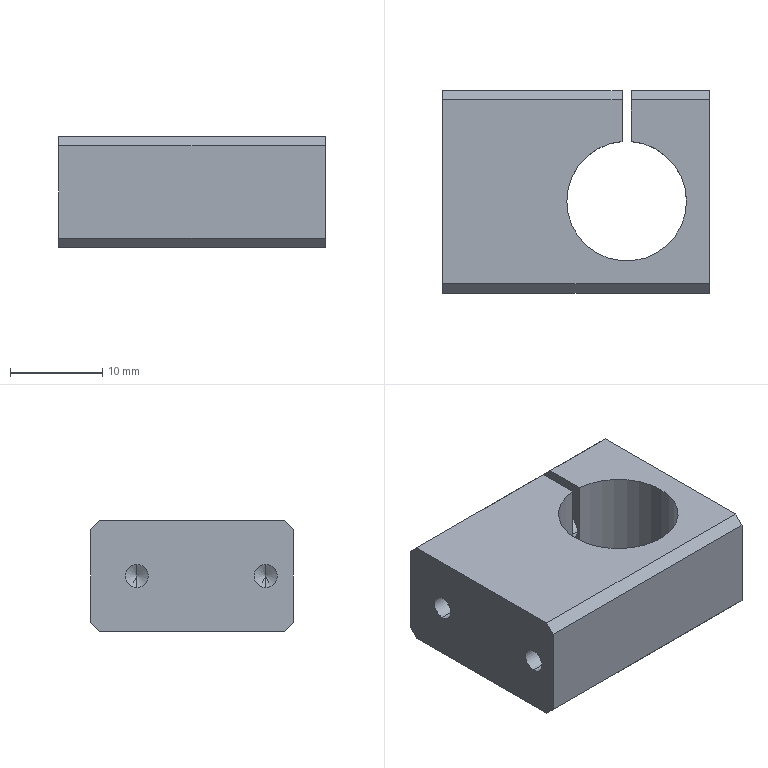Part | NX | 1 solid | 35 faces | box 29 x 22 x 12 mm | volume 5681 mm3 | plane 16 | cylinder 13 | cone 6 | commonest cylinder face diameters 2.5 x6 13 x3 3.4 x2 6 x2
STEP:
#1=CARTESIAN_POINT('',(-3.,7.5,-4.75));
#2=VERTEX_POINT('',#1);
#3=CARTESIAN_POINT('',(-3.,7.5,-7.25));
#4=VERTEX_POINT('',#3);
#5=CARTESIAN_POINT('',(-3.,7.5,-6.));
#6=DIRECTION('',(1.,0.,0.));
#7=DIRECTION('',(0.,0.,-1.));
#8=AXIS2_PLACEMENT_3D('',#5,#6,#7);
#9=CIRCLE('',#8,1.25);
#10=EDGE_CURVE('',#2,#4,#9,.T.);
#11=ORIENTED_EDGE('',*,*,#10,.F.);
#12=CARTESIAN_POINT('',(5.,7.5,-4.75));
#13=VERTEX_POINT('',#12);
#14=CARTESIAN_POINT('',(5.,7.5,-4.75));
#15=DIRECTION('',(1.,0.,0.));
#16=VECTOR('',#15,1000.);
#17=LINE('',#14,#16);
#18=EDGE_CURVE('',#2,#13,#17,.T.);
#19=ORIENTED_EDGE('',*,*,#18,.T.);
#20=CARTESIAN_POINT('',(5.,7.5,-7.25));
#21=VERTEX_POINT('',#20);
#22=CARTESIAN_POINT('',(5.,7.5,-6.));
#23=DIRECTION('',(1.,0.,0.));
#24=DIRECTION('',(0.,0.,-1.));
#25=AXIS2_PLACEMENT_3D('',#22,#23,#24);
#26=CIRCLE('',#25,1.25);
#27=EDGE_CURVE('',#13,#21,#26,.T.);
#28=ORIENTED_EDGE('',*,*,#27,.T.);
#29=CARTESIAN_POINT('',(5.,7.5,-7.25));
#30=DIRECTION('',(1.,0.,0.));
#31=VECTOR('',#30,1000.);
#32=LINE('',#29,#31);
#33=EDGE_CURVE('',#4,#21,#32,.T.);
#34=ORIENTED_EDGE('',*,*,#33,.F.);
#35=EDGE_LOOP('',(#11,#19,#28,#34));
#36=FACE_BOUND('',#35,.T.);
#37=CARTESIAN_POINT('',(5.,7.5,-6.));
#38=DIRECTION('',(1.,0.,0.));
#39=DIRECTION('',(0.,0.,1.));
#40=AXIS2_PLACEMENT_3D('',#37,#38,#39);
#41=CYLINDRICAL_SURFACE('',#40,1.25);
#42=ADVANCED_FACE('',(#36),#41,.F.);
#43=CARTESIAN_POINT('',(-3.751,7.5,-6.));
#44=VERTEX_POINT('',#43);
#45=CARTESIAN_POINT('',(-3.,7.5,-7.25));
#46=DIRECTION('',(0.515,0.,-0.8572));
#47=VECTOR('',#46,1000.);
#48=LINE('',#45,#47);
#49=EDGE_CURVE('',#44,#4,#48,.T.);
#50=ORIENTED_EDGE('',*,*,#49,.F.);
#51=CARTESIAN_POINT('',(-3.,7.5,-4.75));
#52=DIRECTION('',(0.515,0.,0.8572));
#53=VECTOR('',#52,1000.);
#54=LINE('',#51,#53);
#55=EDGE_CURVE('',#44,#2,#54,.T.);
#56=ORIENTED_EDGE('',*,*,#55,.T.);
#57=ORIENTED_EDGE('',*,*,#10,.T.);
#58=EDGE_LOOP('',(#50,#56,#57));
#59=FACE_BOUND('',#58,.T.);
#60=CARTESIAN_POINT('',(-3.,7.5,-6.));
#61=DIRECTION('',(1.,0.,0.));
#62=DIRECTION('',(0.,0.,1.));
#63=AXIS2_PLACEMENT_3D('',#60,#61,#62);
#64=CONICAL_SURFACE('',#63,1.25,1.03);
#65=ADVANCED_FACE('',(#59),#64,.F.);
#66=CARTESIAN_POINT('',(11.1,7.5,-3.));
#67=VERTEX_POINT('',#66);
#68=CARTESIAN_POINT('',(11.1,7.5,-9.));
#69=VERTEX_POINT('',#68);
#70=CARTESIAN_POINT('',(11.1,7.5,-6.));
#71=DIRECTION('',(1.,0.,0.));
#72=DIRECTION('',(0.,0.,-1.));
#73=AXIS2_PLACEMENT_3D('',#70,#71,#72);
#74=CIRCLE('',#73,3.);
#75=EDGE_CURVE('',#67,#69,#74,.T.);
#76=ORIENTED_EDGE('',*,*,#75,.F.);
#77=CARTESIAN_POINT('',(14.5,7.5,-3.));
#78=VERTEX_POINT('',#77);
#79=CARTESIAN_POINT('',(14.5,7.5,-3.));
#80=DIRECTION('',(1.,0.,0.));
#81=VECTOR('',#80,1000.);
#82=LINE('',#79,#81);
#83=EDGE_CURVE('',#67,#78,#82,.T.);
#84=ORIENTED_EDGE('',*,*,#83,.T.);
#85=CARTESIAN_POINT('',(14.5,7.5,-9.));
#86=VERTEX_POINT('',#85);
#87=CARTESIAN_POINT('',(14.5,7.5,-6.));
#88=DIRECTION('',(1.,0.,0.));
#89=DIRECTION('',(0.,0.,-1.));
#90=AXIS2_PLACEMENT_3D('',#87,#88,#89);
#91=CIRCLE('',#90,3.);
#92=EDGE_CURVE('',#78,#86,#91,.T.);
#93=ORIENTED_EDGE('',*,*,#92,.T.);
#94=CARTESIAN_POINT('',(14.5,7.5,-9.));
#95=DIRECTION('',(1.,0.,0.));
#96=VECTOR('',#95,1000.);
#97=LINE('',#94,#96);
#98=EDGE_CURVE('',#69,#86,#97,.T.);
#99=ORIENTED_EDGE('',*,*,#98,.F.);
#100=EDGE_LOOP('',(#76,#84,#93,#99));
#101=FACE_BOUND('',#100,.T.);
#102=CARTESIAN_POINT('',(14.5,7.5,-6.));
#103=DIRECTION('',(1.,0.,0.));
#104=DIRECTION('',(0.,0.,1.));
#105=AXIS2_PLACEMENT_3D('',#102,#103,#104);
#106=CYLINDRICAL_SURFACE('',#105,3.);
#107=ADVANCED_FACE('',(#101),#106,.F.);
#108=CARTESIAN_POINT('',(6.,7.5,-4.3));
#109=VERTEX_POINT('',#108);
#110=CARTESIAN_POINT('',(6.,7.5,-7.7));
#111=VERTEX_POINT('',#110);
#112=CARTESIAN_POINT('',(6.,7.5,-6.));
#113=DIRECTION('',(1.,0.,0.));
#114=DIRECTION('',(0.,1.,0.));
#115=AXIS2_PLACEMENT_3D('',#112,#113,#114);
#116=CIRCLE('',#115,1.7);
#117=EDGE_CURVE('',#109,#111,#116,.T.);
#118=ORIENTED_EDGE('',*,*,#117,.F.);
#119=CARTESIAN_POINT('',(11.1,7.5,-4.3));
#120=VERTEX_POINT('',#119);
#121=CARTESIAN_POINT('',(14.5,7.5,-4.3));
#122=DIRECTION('',(1.,0.,0.));
#123=VECTOR('',#122,1000.);
#124=LINE('',#121,#123);
#125=EDGE_CURVE('',#109,#120,#124,.T.);
#126=ORIENTED_EDGE('',*,*,#125,.T.);
#127=CARTESIAN_POINT('',(11.1,7.5,-7.7));
#128=VERTEX_POINT('',#127);
#129=CARTESIAN_POINT('',(11.1,7.5,-6.));
#130=DIRECTION('',(1.,0.,0.));
#131=DIRECTION('',(0.,0.,-1.));
#132=AXIS2_PLACEMENT_3D('',#129,#130,#131);
#133=CIRCLE('',#132,1.7);
#134=EDGE_CURVE('',#120,#128,#133,.T.);
#135=ORIENTED_EDGE('',*,*,#134,.T.);
#136=CARTESIAN_POINT('',(14.5,7.5,-7.7));
#137=DIRECTION('',(1.,0.,0.));
#138=VECTOR('',#137,1000.);
#139=LINE('',#136,#138);
#140=EDGE_CURVE('',#111,#128,#139,.T.);
#141=ORIENTED_EDGE('',*,*,#140,.F.);
#142=EDGE_LOOP('',(#118,#126,#135,#141));
#143=FACE_BOUND('',#142,.T.);
#144=CARTESIAN_POINT('',(14.5,7.5,-6.));
#145=DIRECTION('',(1.,0.,0.));
#146=DIRECTION('',(0.,0.,1.));
#147=AXIS2_PLACEMENT_3D('',#144,#145,#146);
#148=CYLINDRICAL_SURFACE('',#147,1.7);
#149=ADVANCED_FACE('',(#143),#148,.F.);
#150=CARTESIAN_POINT('',(-7.,6.,-7.25));
#151=VERTEX_POINT('',#150);
#152=CARTESIAN_POINT('',(-7.,6.,-4.75));
#153=VERTEX_POINT('',#152);
#154=CARTESIAN_POINT('',(-7.,6.,-6.));
#155=DIRECTION('',(-1.,0.,0.));
#156=DIRECTION('',(0.,0.,1.));
#157=AXIS2_PLACEMENT_3D('',#154,#155,#156);
#158=CIRCLE('',#157,1.25);
#159=EDGE_CURVE('',#151,#153,#158,.T.);
#160=ORIENTED_EDGE('',*,*,#159,.F.);
#161=CARTESIAN_POINT('',(-14.5,6.,-7.25));
#162=VERTEX_POINT('',#161);
#163=CARTESIAN_POINT('',(-14.5,6.,-7.25));
#164=DIRECTION('',(-1.,0.,0.));
#165=VECTOR('',#164,1000.);
#166=LINE('',#163,#165);
#167=EDGE_CURVE('',#151,#162,#166,.T.);
#168=ORIENTED_EDGE('',*,*,#167,.T.);
#169=CARTESIAN_POINT('',(-14.5,6.,-4.75));
#170=VERTEX_POINT('',#169);
#171=CARTESIAN_POINT('',(-14.5,6.,-6.));
#172=DIRECTION('',(-1.,0.,0.));
#173=DIRECTION('',(0.,0.,1.));
#174=AXIS2_PLACEMENT_3D('',#171,#172,#173);
#175=CIRCLE('',#174,1.25);
#176=EDGE_CURVE('',#162,#170,#175,.T.);
#177=ORIENTED_EDGE('',*,*,#176,.T.);
#178=CARTESIAN_POINT('',(-14.5,6.,-4.75));
#179=DIRECTION('',(-1.,0.,0.));
#180=VECTOR('',#179,1000.);
#181=LINE('',#178,#180);
#182=EDGE_CURVE('',#153,#170,#181,.T.);
#183=ORIENTED_EDGE('',*,*,#182,.F.);
#184=EDGE_LOOP('',(#160,#168,#177,#183));
#185=FACE_BOUND('',#184,.T.);
#186=CARTESIAN_POINT('',(-14.5,6.,-6.));
#187=DIRECTION('',(-1.,0.,0.));
#188=DIRECTION('',(0.,0.,-1.));
#189=AXIS2_PLACEMENT_3D('',#186,#187,#188);
#190=CYLINDRICAL_SURFACE('',#189,1.25);
#191=ADVANCED_FACE('',(#185),#190,.F.);
#192=CARTESIAN_POINT('',(-6.249,6.,-6.));
#193=VERTEX_POINT('',#192);
#194=CARTESIAN_POINT('',(-7.,6.,-4.75));
#195=DIRECTION('',(-0.515,0.,0.8572));
#196=VECTOR('',#195,1000.);
#197=LINE('',#194,#196);
#198=EDGE_CURVE('',#193,#153,#197,.T.);
#199=ORIENTED_EDGE('',*,*,#198,.F.);
#200=CARTESIAN_POINT('',(-7.,6.,-7.25));
#201=DIRECTION('',(-0.515,0.,-0.8572));
#202=VECTOR('',#201,1000.);
#203=LINE('',#200,#202);
#204=EDGE_CURVE('',#193,#151,#203,.T.);
#205=ORIENTED_EDGE('',*,*,#204,.T.);
#206=ORIENTED_EDGE('',*,*,#159,.T.);
#207=EDGE_LOOP('',(#199,#205,#206));
#208=FACE_BOUND('',#207,.T.);
#209=CARTESIAN_POINT('',(-7.,6.,-6.));
#210=DIRECTION('',(-1.,0.,0.));
#211=DIRECTION('',(0.,0.,-1.));
#212=AXIS2_PLACEMENT_3D('',#209,#210,#211);
#213=CONICAL_SURFACE('',#212,1.25,1.03);
#214=ADVANCED_FACE('',(#208),#213,.F.);
#215=CARTESIAN_POINT('',(-7.,-8.,-7.25));
#216=VERTEX_POINT('',#215);
#217=CARTESIAN_POINT('',(-7.,-8.,-4.75));
#218=VERTEX_POINT('',#217);
#219=CARTESIAN_POINT('',(-7.,-8.,-6.));
#220=DIRECTION('',(-1.,0.,0.));
#221=DIRECTION('',(0.,0.,1.));
#222=AXIS2_PLACEMENT_3D('',#219,#220,#221);
#223=CIRCLE('',#222,1.25);
#224=EDGE_CURVE('',#216,#218,#223,.T.);
#225=ORIENTED_EDGE('',*,*,#224,.F.);
#226=CARTESIAN_POINT('',(-14.5,-8.,-7.25));
#227=VERTEX_POINT('',#226);
#228=CARTESIAN_POINT('',(-14.5,-8.,-7.25));
#229=DIRECTION('',(-1.,0.,0.));
#230=VECTOR('',#229,1000.);
#231=LINE('',#228,#230);
#232=EDGE_CURVE('',#216,#227,#231,.T.);
#233=ORIENTED_EDGE('',*,*,#232,.T.);
#234=CARTESIAN_POINT('',(-14.5,-8.,-4.75));
#235=VERTEX_POINT('',#234);
#236=CARTESIAN_POINT('',(-14.5,-8.,-6.));
#237=DIRECTION('',(-1.,0.,0.));
#238=DIRECTION('',(0.,0.,1.));
#239=AXIS2_PLACEMENT_3D('',#236,#237,#238);
#240=CIRCLE('',#239,1.25);
#241=EDGE_CURVE('',#227,#235,#240,.T.);
#242=ORIENTED_EDGE('',*,*,#241,.T.);
#243=CARTESIAN_POINT('',(-14.5,-8.,-4.75));
#244=DIRECTION('',(-1.,0.,0.));
#245=VECTOR('',#244,1000.);
#246=LINE('',#243,#245);
#247=EDGE_CURVE('',#218,#235,#246,.T.);
#248=ORIENTED_EDGE('',*,*,#247,.F.);
#249=EDGE_LOOP('',(#225,#233,#242,#248));
#250=FACE_BOUND('',#249,.T.);
#251=CARTESIAN_POINT('',(-14.5,-8.,-6.));
#252=DIRECTION('',(-1.,0.,0.));
#253=DIRECTION('',(0.,0.,-1.));
#254=AXIS2_PLACEMENT_3D('',#251,#252,#253);
#255=CYLINDRICAL_SURFACE('',#254,1.25);
#256=ADVANCED_FACE('',(#250),#255,.F.);
#257=CARTESIAN_POINT('',(-6.249,-8.,-6.));
#258=VERTEX_POINT('',#257);
#259=CARTESIAN_POINT('',(-7.,-8.,-4.75));
#260=DIRECTION('',(-0.515,0.,0.8572));
#261=VECTOR('',#260,1000.);
#262=LINE('',#259,#261);
#263=EDGE_CURVE('',#258,#218,#262,.T.);
#264=ORIENTED_EDGE('',*,*,#263,.F.);
#265=CARTESIAN_POINT('',(-7.,-8.,-7.25));
#266=DIRECTION('',(-0.515,0.,-0.8572));
#267=VECTOR('',#266,1000.);
#268=LINE('',#265,#267);
#269=EDGE_CURVE('',#258,#216,#268,.T.);
#270=ORIENTED_EDGE('',*,*,#269,.T.);
#271=ORIENTED_EDGE('',*,*,#224,.T.);
#272=EDGE_LOOP('',(#264,#270,#271));
#273=FACE_BOUND('',#272,.T.);
#274=CARTESIAN_POINT('',(-7.,-8.,-6.));
#275=DIRECTION('',(-1.,0.,0.));
#276=DIRECTION('',(0.,0.,-1.));
#277=AXIS2_PLACEMENT_3D('',#274,#275,#276);
#278=CONICAL_SURFACE('',#277,1.25,1.03);
#279=ADVANCED_FACE('',(#273),#278,.F.);
#280=CARTESIAN_POINT('',(-1.,-1.,-12.));
#281=VERTEX_POINT('',#280);
#282=CARTESIAN_POINT('',(12.,-1.,-12.));
#283=VERTEX_POINT('',#282);
#284=CARTESIAN_POINT('',(5.5,-1.,-12.));
#285=DIRECTION('',(0.,0.,1.));
#286=DIRECTION('',(1.,0.,0.));
#287=AXIS2_PLACEMENT_3D('',#284,#285,#286);
#288=CIRCLE('',#287,6.5);
#289=EDGE_CURVE('',#281,#283,#288,.T.);
#290=ORIENTED_EDGE('',*,*,#289,.F.);
#291=CARTESIAN_POINT('',(-1.,-1.,0.));
#292=VERTEX_POINT('',#291);
#293=CARTESIAN_POINT('',(-1.,-1.,-12.));
#294=DIRECTION('',(0.,0.,1.));
#295=VECTOR('',#294,1000.);
#296=LINE('',#293,#295);
#297=EDGE_CURVE('',#281,#292,#296,.T.);
#298=ORIENTED_EDGE('',*,*,#297,.T.);
#299=CARTESIAN_POINT('',(12.,-1.,0.));
#300=VERTEX_POINT('',#299);
#301=CARTESIAN_POINT('',(5.5,-1.,0.));
#302=DIRECTION('',(0.,0.,1.));
#303=DIRECTION('',(1.,0.,0.));
#304=AXIS2_PLACEMENT_3D('',#301,#302,#303);
#305=CIRCLE('',#304,6.5);
#306=EDGE_CURVE('',#292,#300,#305,.T.);
#307=ORIENTED_EDGE('',*,*,#306,.T.);
#308=CARTESIAN_POINT('',(12.,-1.,-12.));
#309=DIRECTION('',(0.,0.,1.));
#310=VECTOR('',#309,1000.);
#311=LINE('',#308,#310);
#312=EDGE_CURVE('',#283,#300,#311,.T.);
#313=ORIENTED_EDGE('',*,*,#312,.F.);
#314=EDGE_LOOP('',(#290,#298,#307,#313));
#315=FACE_BOUND('',#314,.T.);
#316=CARTESIAN_POINT('',(5.5,-1.,-12.));
#317=DIRECTION('',(0.,0.,1.));
#318=DIRECTION('',(-1.,0.,0.));
#319=AXIS2_PLACEMENT_3D('',#316,#317,#318);
#320=CYLINDRICAL_SURFACE('',#319,6.5);
#321=ADVANCED_FACE('',(#315),#320,.F.);
#322=CARTESIAN_POINT('',(6.,5.481,-12.));
#323=VERTEX_POINT('',#322);
#324=CARTESIAN_POINT('',(5.5,-1.,-12.));
#325=DIRECTION('',(0.,0.,1.));
#326=DIRECTION('',(1.,0.,0.));
#327=AXIS2_PLACEMENT_3D('',#324,#325,#326);
#328=CIRCLE('',#327,6.5);
#329=EDGE_CURVE('',#283,#323,#328,.T.);
#330=ORIENTED_EDGE('',*,*,#329,.F.);
#331=ORIENTED_EDGE('',*,*,#312,.T.);
#332=CARTESIAN_POINT('',(6.,5.481,0.));
#333=VERTEX_POINT('',#332);
#334=CARTESIAN_POINT('',(5.5,-1.,0.));
#335=DIRECTION('',(0.,0.,1.));
#336=DIRECTION('',(1.,0.,0.));
#337=AXIS2_PLACEMENT_3D('',#334,#335,#336);
#338=CIRCLE('',#337,6.5);
#339=EDGE_CURVE('',#300,#333,#338,.T.);
#340=ORIENTED_EDGE('',*,*,#339,.T.);
#341=CARTESIAN_POINT('',(6.,5.481,-12.));
#342=DIRECTION('',(0.,0.,1.));
#343=VECTOR('',#342,1000.);
#344=LINE('',#341,#343);
#345=EDGE_CURVE('',#323,#333,#344,.T.);
#346=ORIENTED_EDGE('',*,*,#345,.F.);
#347=EDGE_LOOP('',(#330,#331,#340,#346));
#348=FACE_BOUND('',#347,.T.);
#349=CARTESIAN_POINT('',(5.5,-1.,-12.));
#350=DIRECTION('',(0.,0.,1.));
#351=DIRECTION('',(-1.,0.,0.));
#352=AXIS2_PLACEMENT_3D('',#349,#350,#351);
#353=CYLINDRICAL_SURFACE('',#352,6.5);
#354=ADVANCED_FACE('',(#348),#353,.F.);
#355=CARTESIAN_POINT('',(5.,11.,-11.));
#356=VERTEX_POINT('',#355);
#357=CARTESIAN_POINT('',(5.,11.,-1.));
#358=VERTEX_POINT('',#357);
#359=CARTESIAN_POINT('',(5.,11.,-12.));
#360=DIRECTION('',(0.,0.,1.));
#361=VECTOR('',#360,1000.);
#362=LINE('',#359,#361);
#363=EDGE_CURVE('',#356,#358,#362,.T.);
#364=ORIENTED_EDGE('',*,*,#363,.F.);
#365=CARTESIAN_POINT('',(-14.5,11.,-11.));
#366=VERTEX_POINT('',#365);
#367=CARTESIAN_POINT('',(-14.5,11.,-11.));
#368=DIRECTION('',(-1.,0.,0.));
#369=VECTOR('',#368,1000.);
#370=LINE('',#367,#369);
#371=EDGE_CURVE('',#356,#366,#370,.T.);
#372=ORIENTED_EDGE('',*,*,#371,.T.);
#373=CARTESIAN_POINT('',(-14.5,11.,-1.));
#374=VERTEX_POINT('',#373);
#375=CARTESIAN_POINT('',(-14.5,11.,-12.));
#376=DIRECTION('',(0.,0.,1.));
#377=VECTOR('',#376,1000.);
#378=LINE('',#375,#377);
#379=EDGE_CURVE('',#366,#374,#378,.T.);
#380=ORIENTED_EDGE('',*,*,#379,.T.);
#381=CARTESIAN_POINT('',(5.,11.,-1.));
#382=DIRECTION('',(1.,0.,0.));
#383=VECTOR('',#382,1000.);
#384=LINE('',#381,#383);
#385=EDGE_CURVE('',#374,#358,#384,.T.);
#386=ORIENTED_EDGE('',*,*,#385,.T.);
#387=EDGE_LOOP('',(#364,#372,#380,#386));
#388=FACE_BOUND('',#387,.T.);
#389=CARTESIAN_POINT('',(0.,11.,-6.));
#390=DIRECTION('',(0.,1.,0.));
#391=DIRECTION('',(0.,0.,-1.));
#392=AXIS2_PLACEMENT_3D('',#389,#390,#391);
#393=PLANE('',#392);
#394=ADVANCED_FACE('',(#388),#393,.T.);
#395=CARTESIAN_POINT('',(14.5,7.5,-6.));
#396=DIRECTION('',(1.,0.,0.));
#397=DIRECTION('',(0.,0.,-1.));
#398=AXIS2_PLACEMENT_3D('',#395,#396,#397);
#399=CIRCLE('',#398,3.);
#400=EDGE_CURVE('',#86,#78,#399,.T.);
#401=ORIENTED_EDGE('',*,*,#400,.F.);
#402=ORIENTED_EDGE('',*,*,#92,.F.);
#403=EDGE_LOOP('',(#401,#402));
#404=FACE_BOUND('',#403,.T.);
#405=CARTESIAN_POINT('',(14.5,10.,0.));
#406=VERTEX_POINT('',#405);
#407=CARTESIAN_POINT('',(14.5,-10.,0.));
#408=VERTEX_POINT('',#407);
#409=CARTESIAN_POINT('',(14.5,11.,0.));
#410=DIRECTION('',(0.,-1.,0.));
#411=VECTOR('',#410,1000.);
#412=LINE('',#409,#411);
#413=EDGE_CURVE('',#406,#408,#412,.T.);
#414=ORIENTED_EDGE('',*,*,#413,.T.);
#415=CARTESIAN_POINT('',(14.5,-11.,-1.));
#416=VERTEX_POINT('',#415);
#417=CARTESIAN_POINT('',(14.5,-10.,0.));
#418=DIRECTION('',(0.,-0.7071,-0.7071));
#419=VECTOR('',#418,1000.);
#420=LINE('',#417,#419);
#421=EDGE_CURVE('',#408,#416,#420,.T.);
#422=ORIENTED_EDGE('',*,*,#421,.T.);
#423=CARTESIAN_POINT('',(14.5,-11.,-11.));
#424=VERTEX_POINT('',#423);
#425=CARTESIAN_POINT('',(14.5,-11.,-12.));
#426=DIRECTION('',(0.,0.,-1.));
#427=VECTOR('',#426,1000.);
#428=LINE('',#425,#427);
#429=EDGE_CURVE('',#416,#424,#428,.T.);
#430=ORIENTED_EDGE('',*,*,#429,.T.);
#431=CARTESIAN_POINT('',(14.5,-10.,-12.));
#432=VERTEX_POINT('',#431);
#433=CARTESIAN_POINT('',(14.5,-10.,-12.));
#434=DIRECTION('',(0.,0.7071,-0.7071));
#435=VECTOR('',#434,1000.);
#436=LINE('',#433,#435);
#437=EDGE_CURVE('',#424,#432,#436,.T.);
#438=ORIENTED_EDGE('',*,*,#437,.T.);
#439=CARTESIAN_POINT('',(14.5,10.,-12.));
#440=VERTEX_POINT('',#439);
#441=CARTESIAN_POINT('',(14.5,11.,-12.));
#442=DIRECTION('',(0.,-1.,0.));
#443=VECTOR('',#442,1000.);
#444=LINE('',#441,#443);
#445=EDGE_CURVE('',#440,#432,#444,.T.);
#446=ORIENTED_EDGE('',*,*,#445,.F.);
#447=CARTESIAN_POINT('',(14.5,11.,-11.));
#448=VERTEX_POINT('',#447);
#449=CARTESIAN_POINT('',(14.5,11.,-11.));
#450=DIRECTION('',(0.,0.7071,0.7071));
#451=VECTOR('',#450,1000.);
#452=LINE('',#449,#451);
#453=EDGE_CURVE('',#440,#448,#452,.T.);
#454=ORIENTED_EDGE('',*,*,#453,.T.);
#455=CARTESIAN_POINT('',(14.5,11.,-1.));
#456=VERTEX_POINT('',#455);
#457=CARTESIAN_POINT('',(14.5,11.,-12.));
#458=DIRECTION('',(0.,0.,-1.));
#459=VECTOR('',#458,1000.);
#460=LINE('',#457,#459);
#461=EDGE_CURVE('',#456,#448,#460,.T.);
#462=ORIENTED_EDGE('',*,*,#461,.F.);
#463=CARTESIAN_POINT('',(14.5,11.,-1.));
#464=DIRECTION('',(0.,-0.7071,0.7071));
#465=VECTOR('',#464,1000.);
#466=LINE('',#463,#465);
#467=EDGE_CURVE('',#456,#406,#466,.T.);
#468=ORIENTED_EDGE('',*,*,#467,.T.);
#469=EDGE_LOOP('',(#414,#422,#430,#438,#446,#454,#462,#468));
#470=FACE_BOUND('',#469,.T.);
#471=CARTESIAN_POINT('',(14.5,11.,-12.));
#472=DIRECTION('',(-1.,0.,0.));
#473=DIRECTION('',(0.,0.,-1.));
#474=AXIS2_PLACEMENT_3D('',#471,#472,#473);
#475=PLANE('',#474);
#476=ADVANCED_FACE('',(#404,#470),#475,.F.);
#477=ORIENTED_EDGE('',*,*,#445,.T.);
#478=CARTESIAN_POINT('',(-14.5,-10.,-12.));
#479=VERTEX_POINT('',#478);
#480=CARTESIAN_POINT('',(-14.5,-10.,-12.));
#481=DIRECTION('',(-1.,0.,0.));
#482=VECTOR('',#481,1000.);
#483=LINE('',#480,#482);
#484=EDGE_CURVE('',#432,#479,#483,.T.);
#485=ORIENTED_EDGE('',*,*,#484,.T.);
#486=CARTESIAN_POINT('',(-14.5,10.,-12.));
#487=VERTEX_POINT('',#486);
#488=CARTESIAN_POINT('',(-14.5,11.,-12.));
#489=DIRECTION('',(0.,-1.,0.));
#490=VECTOR('',#489,1000.);
#491=LINE('',#488,#490);
#492=EDGE_CURVE('',#487,#479,#491,.T.);
#493=ORIENTED_EDGE('',*,*,#492,.F.);
#494=CARTESIAN_POINT('',(5.,10.,-12.));
#495=VERTEX_POINT('',#494);
#496=CARTESIAN_POINT('',(5.,10.,-12.));
#497=DIRECTION('',(1.,0.,0.));
#498=VECTOR('',#497,1000.);
#499=LINE('',#496,#498);
#500=EDGE_CURVE('',#487,#495,#499,.T.);
#501=ORIENTED_EDGE('',*,*,#500,.T.);
#502=CARTESIAN_POINT('',(5.,5.481,-12.));
#503=VERTEX_POINT('',#502);
#504=CARTESIAN_POINT('',(5.,5.481,-12.));
#505=DIRECTION('',(0.,-1.,0.));
#506=VECTOR('',#505,1000.);
#507=LINE('',#504,#506);
#508=EDGE_CURVE('',#495,#503,#507,.T.);
#509=ORIENTED_EDGE('',*,*,#508,.T.);
#510=CARTESIAN_POINT('',(5.5,-1.,-12.));
#511=DIRECTION('',(0.,0.,1.));
#512=DIRECTION('',(1.,0.,0.));
#513=AXIS2_PLACEMENT_3D('',#510,#511,#512);
#514=CIRCLE('',#513,6.5);
#515=EDGE_CURVE('',#503,#281,#514,.T.);
#516=ORIENTED_EDGE('',*,*,#515,.T.);
#517=ORIENTED_EDGE('',*,*,#289,.T.);
#518=ORIENTED_EDGE('',*,*,#329,.T.);
#519=CARTESIAN_POINT('',(6.,10.,-12.));
#520=VERTEX_POINT('',#519);
#521=CARTESIAN_POINT('',(6.,11.,-12.));
#522=DIRECTION('',(0.,1.,0.));
#523=VECTOR('',#522,1000.);
#524=LINE('',#521,#523);
#525=EDGE_CURVE('',#323,#520,#524,.T.);
#526=ORIENTED_EDGE('',*,*,#525,.T.);
#527=CARTESIAN_POINT('',(14.5,10.,-12.));
#528=DIRECTION('',(1.,0.,0.));
#529=VECTOR('',#528,1000.);
#530=LINE('',#527,#529);
#531=EDGE_CURVE('',#520,#440,#530,.T.);
#532=ORIENTED_EDGE('',*,*,#531,.T.);
#533=EDGE_LOOP('',(#477,#485,#493,#501,#509,#516,#517,#518,#526,#532));
#534=FACE_BOUND('',#533,.T.);
#535=CARTESIAN_POINT('',(-14.5,11.,-12.));
#536=DIRECTION('',(0.,0.,1.));
#537=DIRECTION('',(-1.,0.,0.));
#538=AXIS2_PLACEMENT_3D('',#535,#536,#537);
#539=PLANE('',#538);
#540=ADVANCED_FACE('',(#534),#539,.F.);
#541=CARTESIAN_POINT('',(-14.5,6.,-6.));
#542=DIRECTION('',(-1.,0.,0.));
#543=DIRECTION('',(0.,0.,1.));
#544=AXIS2_PLACEMENT_3D('',#541,#542,#543);
#545=CIRCLE('',#544,1.25);
#546=EDGE_CURVE('',#170,#162,#545,.T.);
#547=ORIENTED_EDGE('',*,*,#546,.F.);
#548=ORIENTED_EDGE('',*,*,#176,.F.);
#549=EDGE_LOOP('',(#547,#548));
#550=FACE_BOUND('',#549,.T.);
#551=CARTESIAN_POINT('',(-14.5,-8.,-6.));
#552=DIRECTION('',(-1.,0.,0.));
#553=DIRECTION('',(0.,0.,1.));
#554=AXIS2_PLACEMENT_3D('',#551,#552,#553);
#555=CIRCLE('',#554,1.25);
#556=EDGE_CURVE('',#235,#227,#555,.T.);
#557=ORIENTED_EDGE('',*,*,#556,.F.);
#558=ORIENTED_EDGE('',*,*,#241,.F.);
#559=EDGE_LOOP('',(#557,#558));
#560=FACE_BOUND('',#559,.T.);
#561=CARTESIAN_POINT('',(-14.5,-11.,-11.));
#562=VERTEX_POINT('',#561);
#563=CARTESIAN_POINT('',(-14.5,-11.,-1.));
#564=VERTEX_POINT('',#563);
#565=CARTESIAN_POINT('',(-14.5,-11.,-12.));
#566=DIRECTION('',(0.,0.,1.));
#567=VECTOR('',#566,1000.);
#568=LINE('',#565,#567);
#569=EDGE_CURVE('',#562,#564,#568,.T.);
#570=ORIENTED_EDGE('',*,*,#569,.T.);
#571=CARTESIAN_POINT('',(-14.5,-10.,0.));
#572=VERTEX_POINT('',#571);
#573=CARTESIAN_POINT('',(-14.5,-10.,0.));
#574=DIRECTION('',(0.,0.7071,0.7071));
#575=VECTOR('',#574,1000.);
#576=LINE('',#573,#575);
#577=EDGE_CURVE('',#564,#572,#576,.T.);
#578=ORIENTED_EDGE('',*,*,#577,.T.);
#579=CARTESIAN_POINT('',(-14.5,10.,0.));
#580=VERTEX_POINT('',#579);
#581=CARTESIAN_POINT('',(-14.5,11.,0.));
#582=DIRECTION('',(0.,-1.,0.));
#583=VECTOR('',#582,1000.);
#584=LINE('',#581,#583);
#585=EDGE_CURVE('',#580,#572,#584,.T.);
#586=ORIENTED_EDGE('',*,*,#585,.F.);
#587=CARTESIAN_POINT('',(-14.5,11.,-1.));
#588=DIRECTION('',(0.,0.7071,-0.7071));
#589=VECTOR('',#588,1000.);
#590=LINE('',#587,#589);
#591=EDGE_CURVE('',#580,#374,#590,.T.);
#592=ORIENTED_EDGE('',*,*,#591,.T.);
#593=ORIENTED_EDGE('',*,*,#379,.F.);
#594=CARTESIAN_POINT('',(-14.5,11.,-11.));
#595=DIRECTION('',(0.,-0.7071,-0.7071));
#596=VECTOR('',#595,1000.);
#597=LINE('',#594,#596);
#598=EDGE_CURVE('',#366,#487,#597,.T.);
#599=ORIENTED_EDGE('',*,*,#598,.T.);
#600=ORIENTED_EDGE('',*,*,#492,.T.);
#601=CARTESIAN_POINT('',(-14.5,-10.,-12.));
#602=DIRECTION('',(0.,-0.7071,0.7071));
#603=VECTOR('',#602,1000.);
#604=LINE('',#601,#603);
#605=EDGE_CURVE('',#479,#562,#604,.T.);
#606=ORIENTED_EDGE('',*,*,#605,.T.);
#607=EDGE_LOOP('',(#570,#578,#586,#592,#593,#599,#600,#606));
#608=FACE_BOUND('',#607,.T.);
#609=CARTESIAN_POINT('',(-14.5,11.,-12.));
#610=DIRECTION('',(1.,0.,0.));
#611=DIRECTION('',(0.,0.,1.));
#612=AXIS2_PLACEMENT_3D('',#609,#610,#611);
#613=PLANE('',#612);
#614=ADVANCED_FACE('',(#550,#560,#608),#613,.F.);
#615=ORIENTED_EDGE('',*,*,#585,.T.);
#616=CARTESIAN_POINT('',(-14.5,-10.,0.));
#617=DIRECTION('',(1.,0.,0.));
#618=VECTOR('',#617,1000.);
#619=LINE('',#616,#618);
#620=EDGE_CURVE('',#572,#408,#619,.T.);
#621=ORIENTED_EDGE('',*,*,#620,.T.);
#622=ORIENTED_EDGE('',*,*,#413,.F.);
#623=CARTESIAN_POINT('',(6.,10.,0.));
#624=VERTEX_POINT('',#623);
#625=CARTESIAN_POINT('',(6.,10.,0.));
#626=DIRECTION('',(-1.,0.,0.));
#627=VECTOR('',#626,1000.);
#628=LINE('',#625,#627);
#629=EDGE_CURVE('',#406,#624,#628,.T.);
#630=ORIENTED_EDGE('',*,*,#629,.T.);
#631=CARTESIAN_POINT('',(6.,11.,0.));
#632=DIRECTION('',(0.,1.,0.));
#633=VECTOR('',#632,1000.);
#634=LINE('',#631,#633);
#635=EDGE_CURVE('',#333,#624,#634,.T.);
#636=ORIENTED_EDGE('',*,*,#635,.F.);
#637=ORIENTED_EDGE('',*,*,#339,.F.);
#638=ORIENTED_EDGE('',*,*,#306,.F.);
#639=CARTESIAN_POINT('',(5.,5.481,0.));
#640=VERTEX_POINT('',#639);
#641=CARTESIAN_POINT('',(5.5,-1.,0.));
#642=DIRECTION('',(0.,0.,1.));
#643=DIRECTION('',(1.,0.,0.));
#644=AXIS2_PLACEMENT_3D('',#641,#642,#643);
#645=CIRCLE('',#644,6.5);
#646=EDGE_CURVE('',#640,#292,#645,.T.);
#647=ORIENTED_EDGE('',*,*,#646,.F.);
#648=CARTESIAN_POINT('',(5.,10.,0.));
#649=VERTEX_POINT('',#648);
#650=CARTESIAN_POINT('',(5.,5.481,0.));
#651=DIRECTION('',(0.,-1.,0.));
#652=VECTOR('',#651,1000.);
#653=LINE('',#650,#652);
#654=EDGE_CURVE('',#649,#640,#653,.T.);
#655=ORIENTED_EDGE('',*,*,#654,.F.);
#656=CARTESIAN_POINT('',(-14.5,10.,0.));
#657=DIRECTION('',(-1.,0.,0.));
#658=VECTOR('',#657,1000.);
#659=LINE('',#656,#658);
#660=EDGE_CURVE('',#649,#580,#659,.T.);
#661=ORIENTED_EDGE('',*,*,#660,.T.);
#662=EDGE_LOOP('',(#615,#621,#622,#630,#636,#637,#638,#647,#655,#661));
#663=FACE_BOUND('',#662,.T.);
#664=CARTESIAN_POINT('',(-14.5,11.,0.));
#665=DIRECTION('',(0.,0.,-1.));
#666=DIRECTION('',(1.,0.,0.));
#667=AXIS2_PLACEMENT_3D('',#664,#665,#666);
#668=PLANE('',#667);
#669=ADVANCED_FACE('',(#663),#668,.F.);
#670=ORIENTED_EDGE('',*,*,#461,.T.);
#671=CARTESIAN_POINT('',(6.,11.,-11.));
#672=VERTEX_POINT('',#671);
#673=CARTESIAN_POINT('',(6.,11.,-11.));
#674=DIRECTION('',(-1.,0.,0.));
#675=VECTOR('',#674,1000.);
#676=LINE('',#673,#675);
#677=EDGE_CURVE('',#448,#672,#676,.T.);
#678=ORIENTED_EDGE('',*,*,#677,.T.);
#679=CARTESIAN_POINT('',(6.,11.,-1.));
#680=VERTEX_POINT('',#679);
#681=CARTESIAN_POINT('',(6.,11.,-12.));
#682=DIRECTION('',(0.,0.,1.));
#683=VECTOR('',#682,1000.);
#684=LINE('',#681,#683);
#685=EDGE_CURVE('',#672,#680,#684,.T.);
#686=ORIENTED_EDGE('',*,*,#685,.T.);
#687=CARTESIAN_POINT('',(14.5,11.,-1.));
#688=DIRECTION('',(1.,0.,0.));
#689=VECTOR('',#688,1000.);
#690=LINE('',#687,#689);
#691=EDGE_CURVE('',#680,#456,#690,.T.);
#692=ORIENTED_EDGE('',*,*,#691,.T.);
#693=EDGE_LOOP('',(#670,#678,#686,#692));
#694=FACE_BOUND('',#693,.T.);
#695=CARTESIAN_POINT('',(0.,11.,-6.));
#696=DIRECTION('',(0.,1.,0.));
#697=DIRECTION('',(0.,0.,-1.));
#698=AXIS2_PLACEMENT_3D('',#695,#696,#697);
#699=PLANE('',#698);
#700=ADVANCED_FACE('',(#694),#699,.T.);
#701=ORIENTED_EDGE('',*,*,#429,.F.);
#702=CARTESIAN_POINT('',(0.,-11.,-1.));
#703=DIRECTION('',(-1.,0.,0.));
#704=VECTOR('',#703,1000.);
#705=LINE('',#702,#704);
#706=EDGE_CURVE('',#416,#564,#705,.T.);
#707=ORIENTED_EDGE('',*,*,#706,.T.);
#708=ORIENTED_EDGE('',*,*,#569,.F.);
#709=CARTESIAN_POINT('',(0.,-11.,-11.));
#710=DIRECTION('',(1.,0.,0.));
#711=VECTOR('',#710,1000.);
#712=LINE('',#709,#711);
#713=EDGE_CURVE('',#562,#424,#712,.T.);
#714=ORIENTED_EDGE('',*,*,#713,.T.);
#715=EDGE_LOOP('',(#701,#707,#708,#714));
#716=FACE_BOUND('',#715,.T.);
#717=CARTESIAN_POINT('',(0.,-11.,-6.));
#718=DIRECTION('',(0.,1.,0.));
#719=DIRECTION('',(0.,0.,-1.));
#720=AXIS2_PLACEMENT_3D('',#717,#718,#719);
#721=PLANE('',#720);
#722=ADVANCED_FACE('',(#716),#721,.F.);
#723=ORIENTED_EDGE('',*,*,#297,.F.);
#724=ORIENTED_EDGE('',*,*,#515,.F.);
#725=CARTESIAN_POINT('',(5.,5.481,-12.));
#726=DIRECTION('',(0.,0.,1.));
#727=VECTOR('',#726,1000.);
#728=LINE('',#725,#727);
#729=EDGE_CURVE('',#503,#640,#728,.T.);
#730=ORIENTED_EDGE('',*,*,#729,.T.);
#731=ORIENTED_EDGE('',*,*,#646,.T.);
#732=EDGE_LOOP('',(#723,#724,#730,#731));
#733=FACE_BOUND('',#732,.T.);
#734=CARTESIAN_POINT('',(5.5,-1.,-12.));
#735=DIRECTION('',(0.,0.,1.));
#736=DIRECTION('',(-1.,0.,0.));
#737=AXIS2_PLACEMENT_3D('',#734,#735,#736);
#738=CYLINDRICAL_SURFACE('',#737,6.5);
#739=ADVANCED_FACE('',(#733),#738,.F.);
#740=CARTESIAN_POINT('',(5.,7.5,-6.));
#741=DIRECTION('',(1.,0.,0.));
#742=DIRECTION('',(0.,0.,-1.));
#743=AXIS2_PLACEMENT_3D('',#740,#741,#742);
#744=CIRCLE('',#743,1.25);
#745=EDGE_CURVE('',#21,#13,#744,.T.);
#746=ORIENTED_EDGE('',*,*,#745,.F.);
#747=ORIENTED_EDGE('',*,*,#27,.F.);
#748=EDGE_LOOP('',(#746,#747));
#749=FACE_BOUND('',#748,.T.);
#750=ORIENTED_EDGE('',*,*,#508,.F.);
#751=CARTESIAN_POINT('',(5.,11.,-11.));
#752=DIRECTION('',(0.,0.7071,0.7071));
#753=VECTOR('',#752,1000.);
#754=LINE('',#751,#753);
#755=EDGE_CURVE('',#495,#356,#754,.T.);
#756=ORIENTED_EDGE('',*,*,#755,.T.);
#757=ORIENTED_EDGE('',*,*,#363,.T.);
#758=CARTESIAN_POINT('',(5.,11.,-1.));
#759=DIRECTION('',(0.,-0.7071,0.7071));
#760=VECTOR('',#759,1000.);
#761=LINE('',#758,#760);
#762=EDGE_CURVE('',#358,#649,#761,.T.);
#763=ORIENTED_EDGE('',*,*,#762,.T.);
#764=ORIENTED_EDGE('',*,*,#654,.T.);
#765=ORIENTED_EDGE('',*,*,#729,.F.);
#766=EDGE_LOOP('',(#750,#756,#757,#763,#764,#765));
#767=FACE_BOUND('',#766,.T.);
#768=CARTESIAN_POINT('',(5.,5.481,-12.));
#769=DIRECTION('',(-1.,0.,0.));
#770=DIRECTION('',(0.,1.,0.));
#771=AXIS2_PLACEMENT_3D('',#768,#769,#770);
#772=PLANE('',#771);
#773=ADVANCED_FACE('',(#749,#767),#772,.F.);
#774=CARTESIAN_POINT('',(6.,7.5,-6.));
#775=DIRECTION('',(1.,0.,0.));
#776=DIRECTION('',(0.,1.,0.));
#777=AXIS2_PLACEMENT_3D('',#774,#775,#776);
#778=CIRCLE('',#777,1.7);
#779=EDGE_CURVE('',#111,#109,#778,.T.);
#780=ORIENTED_EDGE('',*,*,#779,.T.);
#781=ORIENTED_EDGE('',*,*,#117,.T.);
#782=EDGE_LOOP('',(#780,#781));
#783=FACE_BOUND('',#782,.T.);
#784=ORIENTED_EDGE('',*,*,#685,.F.);
#785=CARTESIAN_POINT('',(6.,11.,-11.));
#786=DIRECTION('',(0.,-0.7071,-0.7071));
#787=VECTOR('',#786,1000.);
#788=LINE('',#785,#787);
#789=EDGE_CURVE('',#672,#520,#788,.T.);
#790=ORIENTED_EDGE('',*,*,#789,.T.);
#791=ORIENTED_EDGE('',*,*,#525,.F.);
#792=ORIENTED_EDGE('',*,*,#345,.T.);
#793=ORIENTED_EDGE('',*,*,#635,.T.);
#794=CARTESIAN_POINT('',(6.,11.,-1.));
#795=DIRECTION('',(0.,0.7071,-0.7071));
#796=VECTOR('',#795,1000.);
#797=LINE('',#794,#796);
#798=EDGE_CURVE('',#624,#680,#797,.T.);
#799=ORIENTED_EDGE('',*,*,#798,.T.);
#800=EDGE_LOOP('',(#784,#790,#791,#792,#793,#799));
#801=FACE_BOUND('',#800,.T.);
#802=CARTESIAN_POINT('',(6.,11.,-12.));
#803=DIRECTION('',(1.,0.,0.));
#804=DIRECTION('',(0.,-1.,0.));
#805=AXIS2_PLACEMENT_3D('',#802,#803,#804);
#806=PLANE('',#805);
#807=ADVANCED_FACE('',(#783,#801),#806,.F.);
#808=ORIENTED_EDGE('',*,*,#269,.F.);
#809=ORIENTED_EDGE('',*,*,#263,.T.);
#810=CARTESIAN_POINT('',(-7.,-8.,-6.));
#811=DIRECTION('',(-1.,0.,0.));
#812=DIRECTION('',(0.,0.,1.));
#813=AXIS2_PLACEMENT_3D('',#810,#811,#812);
#814=CIRCLE('',#813,1.25);
#815=EDGE_CURVE('',#218,#216,#814,.T.);
#816=ORIENTED_EDGE('',*,*,#815,.T.);
#817=EDGE_LOOP('',(#808,#809,#816));
#818=FACE_BOUND('',#817,.T.);
#819=CARTESIAN_POINT('',(-7.,-8.,-6.));
#820=DIRECTION('',(-1.,0.,0.));
#821=DIRECTION('',(0.,0.,-1.));
#822=AXIS2_PLACEMENT_3D('',#819,#820,#821);
#823=CONICAL_SURFACE('',#822,1.25,1.03);
#824=ADVANCED_FACE('',(#818),#823,.F.);
#825=ORIENTED_EDGE('',*,*,#232,.F.);
#826=ORIENTED_EDGE('',*,*,#815,.F.);
#827=ORIENTED_EDGE('',*,*,#247,.T.);
#828=ORIENTED_EDGE('',*,*,#556,.T.);
#829=EDGE_LOOP('',(#825,#826,#827,#828));
#830=FACE_BOUND('',#829,.T.);
#831=CARTESIAN_POINT('',(-14.5,-8.,-6.));
#832=DIRECTION('',(-1.,0.,0.));
#833=DIRECTION('',(0.,0.,-1.));
#834=AXIS2_PLACEMENT_3D('',#831,#832,#833);
#835=CYLINDRICAL_SURFACE('',#834,1.25);
#836=ADVANCED_FACE('',(#830),#835,.F.);
#837=ORIENTED_EDGE('',*,*,#204,.F.);
#838=ORIENTED_EDGE('',*,*,#198,.T.);
#839=CARTESIAN_POINT('',(-7.,6.,-6.));
#840=DIRECTION('',(-1.,0.,0.));
#841=DIRECTION('',(0.,0.,1.));
#842=AXIS2_PLACEMENT_3D('',#839,#840,#841);
#843=CIRCLE('',#842,1.25);
#844=EDGE_CURVE('',#153,#151,#843,.T.);
#845=ORIENTED_EDGE('',*,*,#844,.T.);
#846=EDGE_LOOP('',(#837,#838,#845));
#847=FACE_BOUND('',#846,.T.);
#848=CARTESIAN_POINT('',(-7.,6.,-6.));
#849=DIRECTION('',(-1.,0.,0.));
#850=DIRECTION('',(0.,0.,-1.));
#851=AXIS2_PLACEMENT_3D('',#848,#849,#850);
#852=CONICAL_SURFACE('',#851,1.25,1.03);
#853=ADVANCED_FACE('',(#847),#852,.F.);
#854=ORIENTED_EDGE('',*,*,#167,.F.);
#855=ORIENTED_EDGE('',*,*,#844,.F.);
#856=ORIENTED_EDGE('',*,*,#182,.T.);
#857=ORIENTED_EDGE('',*,*,#546,.T.);
#858=EDGE_LOOP('',(#854,#855,#856,#857));
#859=FACE_BOUND('',#858,.T.);
#860=CARTESIAN_POINT('',(-14.5,6.,-6.));
#861=DIRECTION('',(-1.,0.,0.));
#862=DIRECTION('',(0.,0.,-1.));
#863=AXIS2_PLACEMENT_3D('',#860,#861,#862);
#864=CYLINDRICAL_SURFACE('',#863,1.25);
#865=ADVANCED_FACE('',(#859),#864,.F.);
#866=ORIENTED_EDGE('',*,*,#125,.F.);
#867=ORIENTED_EDGE('',*,*,#779,.F.);
#868=ORIENTED_EDGE('',*,*,#140,.T.);
#869=CARTESIAN_POINT('',(11.1,7.5,-6.));
#870=DIRECTION('',(1.,0.,0.));
#871=DIRECTION('',(0.,0.,-1.));
#872=AXIS2_PLACEMENT_3D('',#869,#870,#871);
#873=CIRCLE('',#872,1.7);
#874=EDGE_CURVE('',#128,#120,#873,.T.);
#875=ORIENTED_EDGE('',*,*,#874,.T.);
#876=EDGE_LOOP('',(#866,#867,#868,#875));
#877=FACE_BOUND('',#876,.T.);
#878=CARTESIAN_POINT('',(14.5,7.5,-6.));
#879=DIRECTION('',(1.,0.,0.));
#880=DIRECTION('',(0.,0.,1.));
#881=AXIS2_PLACEMENT_3D('',#878,#879,#880);
#882=CYLINDRICAL_SURFACE('',#881,1.7);
#883=ADVANCED_FACE('',(#877),#882,.F.);
#884=ORIENTED_EDGE('',*,*,#874,.F.);
#885=ORIENTED_EDGE('',*,*,#134,.F.);
#886=EDGE_LOOP('',(#884,#885));
#887=FACE_BOUND('',#886,.T.);
#888=CARTESIAN_POINT('',(11.1,7.5,-6.));
#889=DIRECTION('',(1.,0.,0.));
#890=DIRECTION('',(0.,0.,-1.));
#891=AXIS2_PLACEMENT_3D('',#888,#889,#890);
#892=CIRCLE('',#891,3.);
#893=EDGE_CURVE('',#69,#67,#892,.T.);
#894=ORIENTED_EDGE('',*,*,#893,.T.);
#895=ORIENTED_EDGE('',*,*,#75,.T.);
#896=EDGE_LOOP('',(#894,#895));
#897=FACE_BOUND('',#896,.T.);
#898=CARTESIAN_POINT('',(11.1,9.2,-6.));
#899=DIRECTION('',(-1.,0.,0.));
#900=DIRECTION('',(0.,0.,-1.));
#901=AXIS2_PLACEMENT_3D('',#898,#899,#900);
#902=PLANE('',#901);
#903=ADVANCED_FACE('',(#887,#897),#902,.F.);
#904=ORIENTED_EDGE('',*,*,#83,.F.);
#905=ORIENTED_EDGE('',*,*,#893,.F.);
#906=ORIENTED_EDGE('',*,*,#98,.T.);
#907=ORIENTED_EDGE('',*,*,#400,.T.);
#908=EDGE_LOOP('',(#904,#905,#906,#907));
#909=FACE_BOUND('',#908,.T.);
#910=CARTESIAN_POINT('',(14.5,7.5,-6.));
#911=DIRECTION('',(1.,0.,0.));
#912=DIRECTION('',(0.,0.,1.));
#913=AXIS2_PLACEMENT_3D('',#910,#911,#912);
#914=CYLINDRICAL_SURFACE('',#913,3.);
#915=ADVANCED_FACE('',(#909),#914,.F.);
#916=ORIENTED_EDGE('',*,*,#55,.F.);
#917=ORIENTED_EDGE('',*,*,#49,.T.);
#918=CARTESIAN_POINT('',(-3.,7.5,-6.));
#919=DIRECTION('',(1.,0.,0.));
#920=DIRECTION('',(0.,0.,-1.));
#921=AXIS2_PLACEMENT_3D('',#918,#919,#920);
#922=CIRCLE('',#921,1.25);
#923=EDGE_CURVE('',#4,#2,#922,.T.);
#924=ORIENTED_EDGE('',*,*,#923,.T.);
#925=EDGE_LOOP('',(#916,#917,#924));
#926=FACE_BOUND('',#925,.T.);
#927=CARTESIAN_POINT('',(-3.,7.5,-6.));
#928=DIRECTION('',(1.,0.,0.));
#929=DIRECTION('',(0.,0.,1.));
#930=AXIS2_PLACEMENT_3D('',#927,#928,#929);
#931=CONICAL_SURFACE('',#930,1.25,1.03);
#932=ADVANCED_FACE('',(#926),#931,.F.);
#933=ORIENTED_EDGE('',*,*,#18,.F.);
#934=ORIENTED_EDGE('',*,*,#923,.F.);
#935=ORIENTED_EDGE('',*,*,#33,.T.);
#936=ORIENTED_EDGE('',*,*,#745,.T.);
#937=EDGE_LOOP('',(#933,#934,#935,#936));
#938=FACE_BOUND('',#937,.T.);
#939=CARTESIAN_POINT('',(5.,7.5,-6.));
#940=DIRECTION('',(1.,0.,0.));
#941=DIRECTION('',(0.,0.,1.));
#942=AXIS2_PLACEMENT_3D('',#939,#940,#941);
#943=CYLINDRICAL_SURFACE('',#942,1.25);
#944=ADVANCED_FACE('',(#938),#943,.F.);
#945=ORIENTED_EDGE('',*,*,#577,.F.);
#946=ORIENTED_EDGE('',*,*,#706,.F.);
#947=ORIENTED_EDGE('',*,*,#421,.F.);
#948=ORIENTED_EDGE('',*,*,#620,.F.);
#949=EDGE_LOOP('',(#945,#946,#947,#948));
#950=FACE_BOUND('',#949,.T.);
#951=CARTESIAN_POINT('',(-14.5,-10.,0.));
#952=DIRECTION('',(0.,0.7071,-0.7071));
#953=DIRECTION('',(-1.,0.,0.));
#954=AXIS2_PLACEMENT_3D('',#951,#952,#953);
#955=PLANE('',#954);
#956=ADVANCED_FACE('',(#950),#955,.F.);
#957=ORIENTED_EDGE('',*,*,#437,.F.);
#958=ORIENTED_EDGE('',*,*,#713,.F.);
#959=ORIENTED_EDGE('',*,*,#605,.F.);
#960=ORIENTED_EDGE('',*,*,#484,.F.);
#961=EDGE_LOOP('',(#957,#958,#959,#960));
#962=FACE_BOUND('',#961,.T.);
#963=CARTESIAN_POINT('',(-14.5,-10.,-12.));
#964=DIRECTION('',(0.,0.7071,0.7071));
#965=DIRECTION('',(1.,0.,0.));
#966=AXIS2_PLACEMENT_3D('',#963,#964,#965);
#967=PLANE('',#966);
#968=ADVANCED_FACE('',(#962),#967,.F.);
#969=ORIENTED_EDGE('',*,*,#453,.F.);
#970=ORIENTED_EDGE('',*,*,#531,.F.);
#971=ORIENTED_EDGE('',*,*,#789,.F.);
#972=ORIENTED_EDGE('',*,*,#677,.F.);
#973=EDGE_LOOP('',(#969,#970,#971,#972));
#974=FACE_BOUND('',#973,.T.);
#975=CARTESIAN_POINT('',(0.,11.,-11.));
#976=DIRECTION('',(0.,0.7071,-0.7071));
#977=DIRECTION('',(-1.,0.,0.));
#978=AXIS2_PLACEMENT_3D('',#975,#976,#977);
#979=PLANE('',#978);
#980=ADVANCED_FACE('',(#974),#979,.T.);
#981=ORIENTED_EDGE('',*,*,#755,.F.);
#982=ORIENTED_EDGE('',*,*,#500,.F.);
#983=ORIENTED_EDGE('',*,*,#598,.F.);
#984=ORIENTED_EDGE('',*,*,#371,.F.);
#985=EDGE_LOOP('',(#981,#982,#983,#984));
#986=FACE_BOUND('',#985,.T.);
#987=CARTESIAN_POINT('',(0.,11.,-11.));
#988=DIRECTION('',(0.,0.7071,-0.7071));
#989=DIRECTION('',(-1.,0.,0.));
#990=AXIS2_PLACEMENT_3D('',#987,#988,#989);
#991=PLANE('',#990);
#992=ADVANCED_FACE('',(#986),#991,.T.);
#993=ORIENTED_EDGE('',*,*,#798,.F.);
#994=ORIENTED_EDGE('',*,*,#629,.F.);
#995=ORIENTED_EDGE('',*,*,#467,.F.);
#996=ORIENTED_EDGE('',*,*,#691,.F.);
#997=EDGE_LOOP('',(#993,#994,#995,#996));
#998=FACE_BOUND('',#997,.T.);
#999=CARTESIAN_POINT('',(0.,11.,-1.));
#1000=DIRECTION('',(0.,0.7071,0.7071));
#1001=DIRECTION('',(1.,0.,0.));
#1002=AXIS2_PLACEMENT_3D('',#999,#1000,#1001);
#1003=PLANE('',#1002);
#1004=ADVANCED_FACE('',(#998),#1003,.T.);
#1005=ORIENTED_EDGE('',*,*,#591,.F.);
#1006=ORIENTED_EDGE('',*,*,#660,.F.);
#1007=ORIENTED_EDGE('',*,*,#762,.F.);
#1008=ORIENTED_EDGE('',*,*,#385,.F.);
#1009=EDGE_LOOP('',(#1005,#1006,#1007,#1008));
#1010=FACE_BOUND('',#1009,.T.);
#1011=CARTESIAN_POINT('',(0.,11.,-1.));
#1012=DIRECTION('',(0.,0.7071,0.7071));
#1013=DIRECTION('',(1.,0.,0.));
#1014=AXIS2_PLACEMENT_3D('',#1011,#1012,#1013);
#1015=PLANE('',#1014);
#1016=ADVANCED_FACE('',(#1010),#1015,.T.);
#1017=CLOSED_SHELL('',(#42,#65,#107,#149,#191,#214,#256,#279,#321,#354,#394,#476,#540,#614,#669,#700,#722,#739,#773,#807,#824,#836,#853,#865,#883,#903,#915,#932,#944,#956,#968,#980,#992,#1004,#1016));
#1018=MANIFOLD_SOLID_BREP('',#1017);
#1019=(LENGTH_UNIT()NAMED_UNIT(*)SI_UNIT(.MILLI.,.METRE.));
#1020=UNCERTAINTY_MEASURE_WITH_UNIT(LENGTH_MEASURE(0.00001),#1019,'','');
#1021=(NAMED_UNIT(*)PLANE_ANGLE_UNIT()SI_UNIT($,.RADIAN.));
#1022=(NAMED_UNIT(*)SI_UNIT($,.STERADIAN.)SOLID_ANGLE_UNIT());
#1023=(GEOMETRIC_REPRESENTATION_CONTEXT(3)GLOBAL_UNCERTAINTY_ASSIGNED_CONTEXT((#1020))GLOBAL_UNIT_ASSIGNED_CONTEXT((#1019,#1021,#1022))REPRESENTATION_CONTEXT('',''));
#1024=ADVANCED_BREP_SHAPE_REPRESENTATION('',(#1018),#1023);